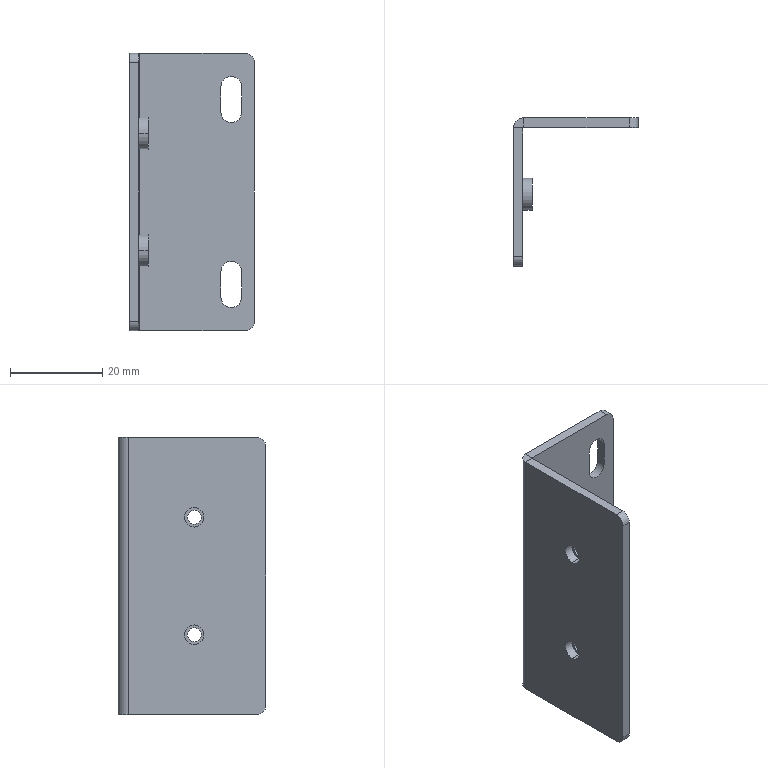Part | STEP file | FBDS-BJ-015 | 1 solid | 44 faces | box 27 x 32 x 60 mm | volume 6673 mm3 | cylinder 24 | plane 20 | commonest cylinder face diameters 4.5 x6 3 x4 4 x4 4.2 x4 6.87 x4 0.4 x1
STEP:
#1=CARTESIAN_POINT('',(2.,-13.,-12.7));
#2=VERTEX_POINT('',#1);
#3=CARTESIAN_POINT('',(2.,-16.,-12.7));
#4=VERTEX_POINT('',#3);
#5=CARTESIAN_POINT('',(2.,-14.5,-12.7));
#6=DIRECTION('',(-1.,0.,0.));
#7=DIRECTION('',(0.,-1.,0.));
#8=AXIS2_PLACEMENT_3D('',#5,#6,#7);
#9=CIRCLE('',#8,1.5);
#10=EDGE_CURVE('',#2,#4,#9,.T.);
#11=ORIENTED_EDGE('',*,*,#10,.F.);
#12=CARTESIAN_POINT('',(0.,-13.,-12.7));
#13=VERTEX_POINT('',#12);
#14=CARTESIAN_POINT('',(2.,-13.,-12.7));
#15=DIRECTION('',(-1.,0.,0.));
#16=VECTOR('',#15,1000.);
#17=LINE('',#14,#16);
#18=EDGE_CURVE('',#2,#13,#17,.T.);
#19=ORIENTED_EDGE('',*,*,#18,.T.);
#20=CARTESIAN_POINT('',(0.,-16.,-12.7));
#21=VERTEX_POINT('',#20);
#22=CARTESIAN_POINT('',(0.,-14.5,-12.7));
#23=DIRECTION('',(-1.,0.,0.));
#24=DIRECTION('',(0.,-1.,0.));
#25=AXIS2_PLACEMENT_3D('',#22,#23,#24);
#26=CIRCLE('',#25,1.5);
#27=EDGE_CURVE('',#13,#21,#26,.T.);
#28=ORIENTED_EDGE('',*,*,#27,.T.);
#29=CARTESIAN_POINT('',(2.,-16.,-12.7));
#30=DIRECTION('',(-1.,0.,0.));
#31=VECTOR('',#30,1000.);
#32=LINE('',#29,#31);
#33=EDGE_CURVE('',#4,#21,#32,.T.);
#34=ORIENTED_EDGE('',*,*,#33,.F.);
#35=EDGE_LOOP('',(#11,#19,#28,#34));
#36=FACE_OUTER_BOUND('',#35,.T.);
#37=CARTESIAN_POINT('',(2.,-14.5,-12.7));
#38=DIRECTION('',(-1.,0.,0.));
#39=DIRECTION('',(0.,-1.,0.));
#40=AXIS2_PLACEMENT_3D('',#37,#38,#39);
#41=CYLINDRICAL_SURFACE('',#40,1.5);
#42=ADVANCED_FACE('',(#36),#41,.F.);
#43=CARTESIAN_POINT('',(2.,-17.935,-12.7));
#44=VERTEX_POINT('',#43);
#45=CARTESIAN_POINT('',(2.,-11.065,-12.7));
#46=VERTEX_POINT('',#45);
#47=CARTESIAN_POINT('',(2.,-14.5,-12.7));
#48=DIRECTION('',(-1.,0.,0.));
#49=DIRECTION('',(0.,0.,1.));
#50=AXIS2_PLACEMENT_3D('',#47,#48,#49);
#51=CIRCLE('',#50,3.435);
#52=EDGE_CURVE('',#44,#46,#51,.T.);
#53=ORIENTED_EDGE('',*,*,#52,.T.);
#54=CARTESIAN_POINT('',(0.,-11.065,-12.7));
#55=VERTEX_POINT('',#54);
#56=CARTESIAN_POINT('',(2.,-11.065,-12.7));
#57=DIRECTION('',(-1.,0.,0.));
#58=VECTOR('',#57,1000.);
#59=LINE('',#56,#58);
#60=EDGE_CURVE('',#46,#55,#59,.T.);
#61=ORIENTED_EDGE('',*,*,#60,.T.);
#62=CARTESIAN_POINT('',(0.,-17.935,-12.7));
#63=VERTEX_POINT('',#62);
#64=CARTESIAN_POINT('',(0.,-14.5,-12.7));
#65=DIRECTION('',(1.,0.,0.));
#66=DIRECTION('',(0.,1.,0.));
#67=AXIS2_PLACEMENT_3D('',#64,#65,#66);
#68=CIRCLE('',#67,3.435);
#69=EDGE_CURVE('',#55,#63,#68,.T.);
#70=ORIENTED_EDGE('',*,*,#69,.T.);
#71=CARTESIAN_POINT('',(2.,-17.935,-12.7));
#72=DIRECTION('',(-1.,0.,0.));
#73=VECTOR('',#72,1000.);
#74=LINE('',#71,#73);
#75=EDGE_CURVE('',#44,#63,#74,.T.);
#76=ORIENTED_EDGE('',*,*,#75,.F.);
#77=EDGE_LOOP('',(#53,#61,#70,#76));
#78=FACE_OUTER_BOUND('',#77,.T.);
#79=CARTESIAN_POINT('',(2.,-14.5,-12.7));
#80=DIRECTION('',(-1.,0.,0.));
#81=DIRECTION('',(0.,-1.,0.));
#82=AXIS2_PLACEMENT_3D('',#79,#80,#81);
#83=CYLINDRICAL_SURFACE('',#82,3.435);
#84=ADVANCED_FACE('',(#78),#83,.T.);
#85=CARTESIAN_POINT('',(2.,-13.,12.7));
#86=VERTEX_POINT('',#85);
#87=CARTESIAN_POINT('',(2.,-16.,12.7));
#88=VERTEX_POINT('',#87);
#89=CARTESIAN_POINT('',(2.,-14.5,12.7));
#90=DIRECTION('',(-1.,0.,0.));
#91=DIRECTION('',(0.,-1.,0.));
#92=AXIS2_PLACEMENT_3D('',#89,#90,#91);
#93=CIRCLE('',#92,1.5);
#94=EDGE_CURVE('',#86,#88,#93,.T.);
#95=ORIENTED_EDGE('',*,*,#94,.F.);
#96=CARTESIAN_POINT('',(0.,-13.,12.7));
#97=VERTEX_POINT('',#96);
#98=CARTESIAN_POINT('',(2.,-13.,12.7));
#99=DIRECTION('',(-1.,0.,0.));
#100=VECTOR('',#99,1000.);
#101=LINE('',#98,#100);
#102=EDGE_CURVE('',#86,#97,#101,.T.);
#103=ORIENTED_EDGE('',*,*,#102,.T.);
#104=CARTESIAN_POINT('',(0.,-16.,12.7));
#105=VERTEX_POINT('',#104);
#106=CARTESIAN_POINT('',(0.,-14.5,12.7));
#107=DIRECTION('',(-1.,0.,0.));
#108=DIRECTION('',(0.,-1.,0.));
#109=AXIS2_PLACEMENT_3D('',#106,#107,#108);
#110=CIRCLE('',#109,1.5);
#111=EDGE_CURVE('',#97,#105,#110,.T.);
#112=ORIENTED_EDGE('',*,*,#111,.T.);
#113=CARTESIAN_POINT('',(2.,-16.,12.7));
#114=DIRECTION('',(-1.,0.,0.));
#115=VECTOR('',#114,1000.);
#116=LINE('',#113,#115);
#117=EDGE_CURVE('',#88,#105,#116,.T.);
#118=ORIENTED_EDGE('',*,*,#117,.F.);
#119=EDGE_LOOP('',(#95,#103,#112,#118));
#120=FACE_OUTER_BOUND('',#119,.T.);
#121=CARTESIAN_POINT('',(2.,-14.5,12.7));
#122=DIRECTION('',(-1.,0.,0.));
#123=DIRECTION('',(0.,-1.,0.));
#124=AXIS2_PLACEMENT_3D('',#121,#122,#123);
#125=CYLINDRICAL_SURFACE('',#124,1.5);
#126=ADVANCED_FACE('',(#120),#125,.F.);
#127=CARTESIAN_POINT('',(2.,-17.935,12.7));
#128=VERTEX_POINT('',#127);
#129=CARTESIAN_POINT('',(2.,-11.065,12.7));
#130=VERTEX_POINT('',#129);
#131=CARTESIAN_POINT('',(2.,-14.5,12.7));
#132=DIRECTION('',(-1.,0.,0.));
#133=DIRECTION('',(0.,0.,1.));
#134=AXIS2_PLACEMENT_3D('',#131,#132,#133);
#135=CIRCLE('',#134,3.435);
#136=EDGE_CURVE('',#128,#130,#135,.T.);
#137=ORIENTED_EDGE('',*,*,#136,.T.);
#138=CARTESIAN_POINT('',(0.,-11.065,12.7));
#139=VERTEX_POINT('',#138);
#140=CARTESIAN_POINT('',(2.,-11.065,12.7));
#141=DIRECTION('',(-1.,0.,0.));
#142=VECTOR('',#141,1000.);
#143=LINE('',#140,#142);
#144=EDGE_CURVE('',#130,#139,#143,.T.);
#145=ORIENTED_EDGE('',*,*,#144,.T.);
#146=CARTESIAN_POINT('',(0.,-17.935,12.7));
#147=VERTEX_POINT('',#146);
#148=CARTESIAN_POINT('',(0.,-14.5,12.7));
#149=DIRECTION('',(1.,0.,0.));
#150=DIRECTION('',(0.,1.,0.));
#151=AXIS2_PLACEMENT_3D('',#148,#149,#150);
#152=CIRCLE('',#151,3.435);
#153=EDGE_CURVE('',#139,#147,#152,.T.);
#154=ORIENTED_EDGE('',*,*,#153,.T.);
#155=CARTESIAN_POINT('',(2.,-17.935,12.7));
#156=DIRECTION('',(-1.,0.,0.));
#157=VECTOR('',#156,1000.);
#158=LINE('',#155,#157);
#159=EDGE_CURVE('',#128,#147,#158,.T.);
#160=ORIENTED_EDGE('',*,*,#159,.F.);
#161=EDGE_LOOP('',(#137,#145,#154,#160));
#162=FACE_OUTER_BOUND('',#161,.T.);
#163=CARTESIAN_POINT('',(2.,-14.5,12.7));
#164=DIRECTION('',(-1.,0.,0.));
#165=DIRECTION('',(0.,-1.,0.));
#166=AXIS2_PLACEMENT_3D('',#163,#164,#165);
#167=CYLINDRICAL_SURFACE('',#166,3.435);
#168=ADVANCED_FACE('',(#162),#167,.T.);
#169=CARTESIAN_POINT('',(22.25,0.,22.75));
#170=VERTEX_POINT('',#169);
#171=CARTESIAN_POINT('',(20.,0.,25.));
#172=VERTEX_POINT('',#171);
#173=CARTESIAN_POINT('',(20.,0.,22.75));
#174=DIRECTION('',(0.,-1.,0.));
#175=DIRECTION('',(0.,0.,-1.));
#176=AXIS2_PLACEMENT_3D('',#173,#174,#175);
#177=CIRCLE('',#176,2.25);
#178=EDGE_CURVE('',#170,#172,#177,.T.);
#179=ORIENTED_EDGE('',*,*,#178,.T.);
#180=CARTESIAN_POINT('',(20.,2.,25.));
#181=VERTEX_POINT('',#180);
#182=CARTESIAN_POINT('',(20.,2.,25.));
#183=DIRECTION('',(0.,1.,0.));
#184=VECTOR('',#183,1000.);
#185=LINE('',#182,#184);
#186=EDGE_CURVE('',#172,#181,#185,.T.);
#187=ORIENTED_EDGE('',*,*,#186,.T.);
#188=CARTESIAN_POINT('',(22.25,2.,22.75));
#189=VERTEX_POINT('',#188);
#190=CARTESIAN_POINT('',(20.,2.,22.75));
#191=DIRECTION('',(0.,1.,0.));
#192=DIRECTION('',(0.,0.,1.));
#193=AXIS2_PLACEMENT_3D('',#190,#191,#192);
#194=CIRCLE('',#193,2.25);
#195=EDGE_CURVE('',#181,#189,#194,.T.);
#196=ORIENTED_EDGE('',*,*,#195,.T.);
#197=CARTESIAN_POINT('',(22.25,-8.1,22.75));
#198=DIRECTION('',(0.,-1.,0.));
#199=VECTOR('',#198,1000.);
#200=LINE('',#197,#199);
#201=EDGE_CURVE('',#189,#170,#200,.T.);
#202=ORIENTED_EDGE('',*,*,#201,.T.);
#203=EDGE_LOOP('',(#179,#187,#196,#202));
#204=FACE_OUTER_BOUND('',#203,.T.);
#205=CARTESIAN_POINT('',(20.,2.,22.75));
#206=DIRECTION('',(0.,1.,0.));
#207=DIRECTION('',(0.,0.,1.));
#208=AXIS2_PLACEMENT_3D('',#205,#206,#207);
#209=CYLINDRICAL_SURFACE('',#208,2.25);
#210=ADVANCED_FACE('',(#204),#209,.F.);
#211=CARTESIAN_POINT('',(22.25,0.,-17.25));
#212=VERTEX_POINT('',#211);
#213=CARTESIAN_POINT('',(20.,0.,-15.));
#214=VERTEX_POINT('',#213);
#215=CARTESIAN_POINT('',(20.,0.,-17.25));
#216=DIRECTION('',(0.,-1.,0.));
#217=DIRECTION('',(0.,0.,-1.));
#218=AXIS2_PLACEMENT_3D('',#215,#216,#217);
#219=CIRCLE('',#218,2.25);
#220=EDGE_CURVE('',#212,#214,#219,.T.);
#221=ORIENTED_EDGE('',*,*,#220,.T.);
#222=CARTESIAN_POINT('',(20.,2.,-15.));
#223=VERTEX_POINT('',#222);
#224=CARTESIAN_POINT('',(20.,2.,-15.));
#225=DIRECTION('',(0.,1.,0.));
#226=VECTOR('',#225,1000.);
#227=LINE('',#224,#226);
#228=EDGE_CURVE('',#214,#223,#227,.T.);
#229=ORIENTED_EDGE('',*,*,#228,.T.);
#230=CARTESIAN_POINT('',(22.25,2.,-17.25));
#231=VERTEX_POINT('',#230);
#232=CARTESIAN_POINT('',(20.,2.,-17.25));
#233=DIRECTION('',(0.,1.,0.));
#234=DIRECTION('',(0.,0.,1.));
#235=AXIS2_PLACEMENT_3D('',#232,#233,#234);
#236=CIRCLE('',#235,2.25);
#237=EDGE_CURVE('',#223,#231,#236,.T.);
#238=ORIENTED_EDGE('',*,*,#237,.T.);
#239=CARTESIAN_POINT('',(22.25,-8.1,-17.25));
#240=DIRECTION('',(0.,-1.,0.));
#241=VECTOR('',#240,1000.);
#242=LINE('',#239,#241);
#243=EDGE_CURVE('',#231,#212,#242,.T.);
#244=ORIENTED_EDGE('',*,*,#243,.T.);
#245=EDGE_LOOP('',(#221,#229,#238,#244));
#246=FACE_OUTER_BOUND('',#245,.T.);
#247=CARTESIAN_POINT('',(20.,2.,-17.25));
#248=DIRECTION('',(0.,1.,0.));
#249=DIRECTION('',(0.,0.,1.));
#250=AXIS2_PLACEMENT_3D('',#247,#248,#249);
#251=CYLINDRICAL_SURFACE('',#250,2.25);
#252=ADVANCED_FACE('',(#246),#251,.F.);
#253=CARTESIAN_POINT('',(0.,-14.5,14.8));
#254=VERTEX_POINT('',#253);
#255=CARTESIAN_POINT('',(0.,-14.5,10.6));
#256=VERTEX_POINT('',#255);
#257=CARTESIAN_POINT('',(0.,-14.5,12.7));
#258=DIRECTION('',(1.,0.,0.));
#259=DIRECTION('',(0.,-1.,0.));
#260=AXIS2_PLACEMENT_3D('',#257,#258,#259);
#261=CIRCLE('',#260,2.1);
#262=EDGE_CURVE('',#254,#256,#261,.T.);
#263=ORIENTED_EDGE('',*,*,#262,.T.);
#264=CARTESIAN_POINT('',(-2.,-14.5,10.6));
#265=VERTEX_POINT('',#264);
#266=CARTESIAN_POINT('',(-2.,-14.5,10.6));
#267=DIRECTION('',(-1.,0.,0.));
#268=VECTOR('',#267,1000.);
#269=LINE('',#266,#268);
#270=EDGE_CURVE('',#256,#265,#269,.T.);
#271=ORIENTED_EDGE('',*,*,#270,.T.);
#272=CARTESIAN_POINT('',(-2.,-14.5,14.8));
#273=VERTEX_POINT('',#272);
#274=CARTESIAN_POINT('',(-2.,-14.5,12.7));
#275=DIRECTION('',(-1.,0.,0.));
#276=DIRECTION('',(0.,0.,1.));
#277=AXIS2_PLACEMENT_3D('',#274,#275,#276);
#278=CIRCLE('',#277,2.1);
#279=EDGE_CURVE('',#265,#273,#278,.T.);
#280=ORIENTED_EDGE('',*,*,#279,.T.);
#281=CARTESIAN_POINT('',(-2.,-14.5,14.8));
#282=DIRECTION('',(-1.,0.,0.));
#283=VECTOR('',#282,1000.);
#284=LINE('',#281,#283);
#285=EDGE_CURVE('',#254,#273,#284,.T.);
#286=ORIENTED_EDGE('',*,*,#285,.F.);
#287=EDGE_LOOP('',(#263,#271,#280,#286));
#288=FACE_OUTER_BOUND('',#287,.T.);
#289=CARTESIAN_POINT('',(-2.,-14.5,12.7));
#290=DIRECTION('',(-1.,0.,0.));
#291=DIRECTION('',(0.,0.,1.));
#292=AXIS2_PLACEMENT_3D('',#289,#290,#291);
#293=CYLINDRICAL_SURFACE('',#292,2.1);
#294=ADVANCED_FACE('',(#288),#293,.F.);
#295=CARTESIAN_POINT('',(0.,-14.5,-10.6));
#296=VERTEX_POINT('',#295);
#297=CARTESIAN_POINT('',(0.,-14.5,-14.8));
#298=VERTEX_POINT('',#297);
#299=CARTESIAN_POINT('',(0.,-14.5,-12.7));
#300=DIRECTION('',(1.,0.,0.));
#301=DIRECTION('',(0.,-1.,0.));
#302=AXIS2_PLACEMENT_3D('',#299,#300,#301);
#303=CIRCLE('',#302,2.1);
#304=EDGE_CURVE('',#296,#298,#303,.T.);
#305=ORIENTED_EDGE('',*,*,#304,.T.);
#306=CARTESIAN_POINT('',(-2.,-14.5,-14.8));
#307=VERTEX_POINT('',#306);
#308=CARTESIAN_POINT('',(-2.,-14.5,-14.8));
#309=DIRECTION('',(-1.,0.,0.));
#310=VECTOR('',#309,1000.);
#311=LINE('',#308,#310);
#312=EDGE_CURVE('',#298,#307,#311,.T.);
#313=ORIENTED_EDGE('',*,*,#312,.T.);
#314=CARTESIAN_POINT('',(-2.,-14.5,-10.6));
#315=VERTEX_POINT('',#314);
#316=CARTESIAN_POINT('',(-2.,-14.5,-12.7));
#317=DIRECTION('',(-1.,0.,0.));
#318=DIRECTION('',(0.,0.,1.));
#319=AXIS2_PLACEMENT_3D('',#316,#317,#318);
#320=CIRCLE('',#319,2.1);
#321=EDGE_CURVE('',#307,#315,#320,.T.);
#322=ORIENTED_EDGE('',*,*,#321,.T.);
#323=CARTESIAN_POINT('',(-2.,-14.5,-10.6));
#324=DIRECTION('',(-1.,0.,0.));
#325=VECTOR('',#324,1000.);
#326=LINE('',#323,#325);
#327=EDGE_CURVE('',#296,#315,#326,.T.);
#328=ORIENTED_EDGE('',*,*,#327,.F.);
#329=EDGE_LOOP('',(#305,#313,#322,#328));
#330=FACE_OUTER_BOUND('',#329,.T.);
#331=CARTESIAN_POINT('',(-2.,-14.5,-12.7));
#332=DIRECTION('',(-1.,0.,0.));
#333=DIRECTION('',(0.,0.,1.));
#334=AXIS2_PLACEMENT_3D('',#331,#332,#333);
#335=CYLINDRICAL_SURFACE('',#334,2.1);
#336=ADVANCED_FACE('',(#330),#335,.F.);
#337=CARTESIAN_POINT('',(17.75,2.,22.75));
#338=VERTEX_POINT('',#337);
#339=CARTESIAN_POINT('',(17.75,2.,17.25));
#340=VERTEX_POINT('',#339);
#341=CARTESIAN_POINT('',(17.75,2.,22.75));
#342=DIRECTION('',(0.,0.,-1.));
#343=VECTOR('',#342,1000.);
#344=LINE('',#341,#343);
#345=EDGE_CURVE('',#338,#340,#344,.T.);
#346=ORIENTED_EDGE('',*,*,#345,.T.);
#347=CARTESIAN_POINT('',(22.25,2.,17.25));
#348=VERTEX_POINT('',#347);
#349=CARTESIAN_POINT('',(20.,2.,17.25));
#350=DIRECTION('',(0.,1.,0.));
#351=DIRECTION('',(0.,0.,1.));
#352=AXIS2_PLACEMENT_3D('',#349,#350,#351);
#353=CIRCLE('',#352,2.25);
#354=EDGE_CURVE('',#348,#340,#353,.T.);
#355=ORIENTED_EDGE('',*,*,#354,.F.);
#356=CARTESIAN_POINT('',(22.25,2.,22.75));
#357=DIRECTION('',(0.,0.,-1.));
#358=VECTOR('',#357,1000.);
#359=LINE('',#356,#358);
#360=EDGE_CURVE('',#189,#348,#359,.T.);
#361=ORIENTED_EDGE('',*,*,#360,.F.);
#362=ORIENTED_EDGE('',*,*,#195,.F.);
#363=CARTESIAN_POINT('',(20.,2.,22.75));
#364=DIRECTION('',(0.,1.,0.));
#365=DIRECTION('',(0.,0.,1.));
#366=AXIS2_PLACEMENT_3D('',#363,#364,#365);
#367=CIRCLE('',#366,2.25);
#368=EDGE_CURVE('',#338,#181,#367,.T.);
#369=ORIENTED_EDGE('',*,*,#368,.F.);
#370=EDGE_LOOP('',(#346,#355,#361,#362,#369));
#371=FACE_BOUND('',#370,.T.);
#372=CARTESIAN_POINT('',(25.,2.,28.));
#373=VERTEX_POINT('',#372);
#374=CARTESIAN_POINT('',(25.,2.,-28.));
#375=VERTEX_POINT('',#374);
#376=CARTESIAN_POINT('',(25.,2.,30.));
#377=DIRECTION('',(0.,0.,-1.));
#378=VECTOR('',#377,1000.);
#379=LINE('',#376,#378);
#380=EDGE_CURVE('',#373,#375,#379,.T.);
#381=ORIENTED_EDGE('',*,*,#380,.T.);
#382=CARTESIAN_POINT('',(23.,2.,-30.));
#383=VERTEX_POINT('',#382);
#384=CARTESIAN_POINT('',(23.,2.,-28.));
#385=DIRECTION('',(0.,1.,0.));
#386=DIRECTION('',(0.,0.,-1.));
#387=AXIS2_PLACEMENT_3D('',#384,#385,#386);
#388=CIRCLE('',#387,2.);
#389=EDGE_CURVE('',#375,#383,#388,.T.);
#390=ORIENTED_EDGE('',*,*,#389,.T.);
#391=CARTESIAN_POINT('',(0.2,2.,-30.));
#392=VERTEX_POINT('',#391);
#393=CARTESIAN_POINT('',(0.,2.,-30.));
#394=DIRECTION('',(-1.,0.,0.));
#395=VECTOR('',#394,1000.);
#396=LINE('',#393,#395);
#397=EDGE_CURVE('',#383,#392,#396,.T.);
#398=ORIENTED_EDGE('',*,*,#397,.T.);
#399=CARTESIAN_POINT('',(0.2,2.,30.));
#400=VERTEX_POINT('',#399);
#401=CARTESIAN_POINT('',(0.2,2.,30.));
#402=DIRECTION('',(0.,0.,-1.));
#403=VECTOR('',#402,1000.);
#404=LINE('',#401,#403);
#405=EDGE_CURVE('',#400,#392,#404,.T.);
#406=ORIENTED_EDGE('',*,*,#405,.F.);
#407=CARTESIAN_POINT('',(23.,2.,30.));
#408=VERTEX_POINT('',#407);
#409=CARTESIAN_POINT('',(0.,2.,30.));
#410=DIRECTION('',(-1.,0.,0.));
#411=VECTOR('',#410,1000.);
#412=LINE('',#409,#411);
#413=EDGE_CURVE('',#408,#400,#412,.T.);
#414=ORIENTED_EDGE('',*,*,#413,.F.);
#415=CARTESIAN_POINT('',(23.,2.,28.));
#416=DIRECTION('',(0.,1.,0.));
#417=DIRECTION('',(0.,0.,-1.));
#418=AXIS2_PLACEMENT_3D('',#415,#416,#417);
#419=CIRCLE('',#418,2.);
#420=EDGE_CURVE('',#408,#373,#419,.T.);
#421=ORIENTED_EDGE('',*,*,#420,.T.);
#422=EDGE_LOOP('',(#381,#390,#398,#406,#414,#421));
#423=FACE_OUTER_BOUND('',#422,.T.);
#424=CARTESIAN_POINT('',(22.25,2.,-22.75));
#425=VERTEX_POINT('',#424);
#426=CARTESIAN_POINT('',(17.75,2.,-22.75));
#427=VERTEX_POINT('',#426);
#428=CARTESIAN_POINT('',(20.,2.,-22.75));
#429=DIRECTION('',(0.,1.,0.));
#430=DIRECTION('',(0.,0.,1.));
#431=AXIS2_PLACEMENT_3D('',#428,#429,#430);
#432=CIRCLE('',#431,2.25);
#433=EDGE_CURVE('',#425,#427,#432,.T.);
#434=ORIENTED_EDGE('',*,*,#433,.F.);
#435=CARTESIAN_POINT('',(22.25,2.,-17.25));
#436=DIRECTION('',(0.,0.,-1.));
#437=VECTOR('',#436,1000.);
#438=LINE('',#435,#437);
#439=EDGE_CURVE('',#231,#425,#438,.T.);
#440=ORIENTED_EDGE('',*,*,#439,.F.);
#441=ORIENTED_EDGE('',*,*,#237,.F.);
#442=CARTESIAN_POINT('',(17.75,2.,-17.25));
#443=VERTEX_POINT('',#442);
#444=CARTESIAN_POINT('',(20.,2.,-17.25));
#445=DIRECTION('',(0.,1.,0.));
#446=DIRECTION('',(0.,0.,1.));
#447=AXIS2_PLACEMENT_3D('',#444,#445,#446);
#448=CIRCLE('',#447,2.25);
#449=EDGE_CURVE('',#443,#223,#448,.T.);
#450=ORIENTED_EDGE('',*,*,#449,.F.);
#451=CARTESIAN_POINT('',(17.75,2.,-17.25));
#452=DIRECTION('',(0.,0.,-1.));
#453=VECTOR('',#452,1000.);
#454=LINE('',#451,#453);
#455=EDGE_CURVE('',#443,#427,#454,.T.);
#456=ORIENTED_EDGE('',*,*,#455,.T.);
#457=EDGE_LOOP('',(#434,#440,#441,#450,#456));
#458=FACE_BOUND('',#457,.T.);
#459=CARTESIAN_POINT('',(0.,2.,30.));
#460=DIRECTION('',(0.,-1.,0.));
#461=DIRECTION('',(0.,0.,-1.));
#462=AXIS2_PLACEMENT_3D('',#459,#460,#461);
#463=PLANE('',#462);
#464=ADVANCED_FACE('',(#371,#423,#458),#463,.F.);
#465=CARTESIAN_POINT('',(0.,-0.2,30.));
#466=VERTEX_POINT('',#465);
#467=CARTESIAN_POINT('',(-2.,-0.2,30.));
#468=VERTEX_POINT('',#467);
#469=CARTESIAN_POINT('',(0.,-0.2,30.));
#470=DIRECTION('',(-1.,0.,0.));
#471=VECTOR('',#470,1000.);
#472=LINE('',#469,#471);
#473=EDGE_CURVE('',#466,#468,#472,.T.);
#474=ORIENTED_EDGE('',*,*,#473,.F.);
#475=CARTESIAN_POINT('',(0.2,0.,30.));
#476=VERTEX_POINT('',#475);
#477=CARTESIAN_POINT('',(0.2,-0.2,30.));
#478=DIRECTION('',(0.,0.,1.));
#479=DIRECTION('',(-1.,0.,0.));
#480=AXIS2_PLACEMENT_3D('',#477,#478,#479);
#481=CIRCLE('',#480,0.2);
#482=EDGE_CURVE('',#476,#466,#481,.T.);
#483=ORIENTED_EDGE('',*,*,#482,.F.);
#484=CARTESIAN_POINT('',(0.2,2.,30.));
#485=DIRECTION('',(0.,-1.,0.));
#486=VECTOR('',#485,1000.);
#487=LINE('',#484,#486);
#488=EDGE_CURVE('',#400,#476,#487,.T.);
#489=ORIENTED_EDGE('',*,*,#488,.F.);
#490=CARTESIAN_POINT('',(0.2,-0.2,30.));
#491=DIRECTION('',(0.,0.,1.));
#492=DIRECTION('',(1.,0.,0.));
#493=AXIS2_PLACEMENT_3D('',#490,#491,#492);
#494=CIRCLE('',#493,2.2);
#495=EDGE_CURVE('',#400,#468,#494,.T.);
#496=ORIENTED_EDGE('',*,*,#495,.T.);
#497=EDGE_LOOP('',(#474,#483,#489,#496));
#498=FACE_OUTER_BOUND('',#497,.T.);
#499=CARTESIAN_POINT('',(0.,-0.2,30.));
#500=DIRECTION('',(0.,0.,1.));
#501=DIRECTION('',(1.,0.,0.));
#502=AXIS2_PLACEMENT_3D('',#499,#500,#501);
#503=PLANE('',#502);
#504=ADVANCED_FACE('',(#498),#503,.T.);
#505=CARTESIAN_POINT('',(-2.,-28.,30.));
#506=VERTEX_POINT('',#505);
#507=CARTESIAN_POINT('',(-2.,0.,30.));
#508=DIRECTION('',(0.,-1.,0.));
#509=VECTOR('',#508,1000.);
#510=LINE('',#507,#509);
#511=EDGE_CURVE('',#468,#506,#510,.T.);
#512=ORIENTED_EDGE('',*,*,#511,.T.);
#513=CARTESIAN_POINT('',(0.,-28.,30.));
#514=VERTEX_POINT('',#513);
#515=CARTESIAN_POINT('',(0.2,-28.,30.));
#516=DIRECTION('',(1.,0.,0.));
#517=VECTOR('',#516,1000.);
#518=LINE('',#515,#517);
#519=EDGE_CURVE('',#506,#514,#518,.T.);
#520=ORIENTED_EDGE('',*,*,#519,.T.);
#521=CARTESIAN_POINT('',(0.,0.,30.));
#522=DIRECTION('',(0.,-1.,0.));
#523=VECTOR('',#522,1000.);
#524=LINE('',#521,#523);
#525=EDGE_CURVE('',#466,#514,#524,.T.);
#526=ORIENTED_EDGE('',*,*,#525,.F.);
#527=ORIENTED_EDGE('',*,*,#473,.T.);
#528=EDGE_LOOP('',(#512,#520,#526,#527));
#529=FACE_OUTER_BOUND('',#528,.T.);
#530=CARTESIAN_POINT('',(0.2,2.,30.));
#531=DIRECTION('',(0.,0.,1.));
#532=DIRECTION('',(1.,0.,0.));
#533=AXIS2_PLACEMENT_3D('',#530,#531,#532);
#534=PLANE('',#533);
#535=ADVANCED_FACE('',(#529),#534,.T.);
#536=CARTESIAN_POINT('',(0.2,0.,-30.));
#537=VERTEX_POINT('',#536);
#538=CARTESIAN_POINT('',(0.2,0.,-30.));
#539=DIRECTION('',(0.,1.,0.));
#540=VECTOR('',#539,1000.);
#541=LINE('',#538,#540);
#542=EDGE_CURVE('',#537,#392,#541,.T.);
#543=ORIENTED_EDGE('',*,*,#542,.F.);
#544=CARTESIAN_POINT('',(0.,-0.2,-30.));
#545=VERTEX_POINT('',#544);
#546=CARTESIAN_POINT('',(0.2,-0.2,-30.));
#547=DIRECTION('',(0.,0.,1.));
#548=DIRECTION('',(-1.,0.,0.));
#549=AXIS2_PLACEMENT_3D('',#546,#547,#548);
#550=CIRCLE('',#549,0.2);
#551=EDGE_CURVE('',#537,#545,#550,.T.);
#552=ORIENTED_EDGE('',*,*,#551,.T.);
#553=CARTESIAN_POINT('',(-2.,-0.2,-30.));
#554=VERTEX_POINT('',#553);
#555=CARTESIAN_POINT('',(-2.,-0.2,-30.));
#556=DIRECTION('',(1.,0.,0.));
#557=VECTOR('',#556,1000.);
#558=LINE('',#555,#557);
#559=EDGE_CURVE('',#554,#545,#558,.T.);
#560=ORIENTED_EDGE('',*,*,#559,.F.);
#561=CARTESIAN_POINT('',(0.2,-0.2,-30.));
#562=DIRECTION('',(0.,0.,1.));
#563=DIRECTION('',(1.,0.,0.));
#564=AXIS2_PLACEMENT_3D('',#561,#562,#563);
#565=CIRCLE('',#564,2.2);
#566=EDGE_CURVE('',#392,#554,#565,.T.);
#567=ORIENTED_EDGE('',*,*,#566,.F.);
#568=EDGE_LOOP('',(#543,#552,#560,#567));
#569=FACE_OUTER_BOUND('',#568,.T.);
#570=CARTESIAN_POINT('',(0.2,0.,-30.));
#571=DIRECTION('',(0.,0.,-1.));
#572=DIRECTION('',(-1.,0.,0.));
#573=AXIS2_PLACEMENT_3D('',#570,#571,#572);
#574=PLANE('',#573);
#575=ADVANCED_FACE('',(#569),#574,.T.);
#576=ORIENTED_EDGE('',*,*,#397,.F.);
#577=CARTESIAN_POINT('',(23.,0.,-30.));
#578=VERTEX_POINT('',#577);
#579=CARTESIAN_POINT('',(23.,-0.2,-30.));
#580=DIRECTION('',(0.,-1.,0.));
#581=VECTOR('',#580,1000.);
#582=LINE('',#579,#581);
#583=EDGE_CURVE('',#383,#578,#582,.T.);
#584=ORIENTED_EDGE('',*,*,#583,.T.);
#585=CARTESIAN_POINT('',(0.,0.,-30.));
#586=DIRECTION('',(-1.,0.,0.));
#587=VECTOR('',#586,1000.);
#588=LINE('',#585,#587);
#589=EDGE_CURVE('',#578,#537,#588,.T.);
#590=ORIENTED_EDGE('',*,*,#589,.T.);
#591=ORIENTED_EDGE('',*,*,#542,.T.);
#592=EDGE_LOOP('',(#576,#584,#590,#591));
#593=FACE_OUTER_BOUND('',#592,.T.);
#594=CARTESIAN_POINT('',(-2.,-0.2,-30.));
#595=DIRECTION('',(0.,0.,-1.));
#596=DIRECTION('',(-1.,0.,0.));
#597=AXIS2_PLACEMENT_3D('',#594,#595,#596);
#598=PLANE('',#597);
#599=ADVANCED_FACE('',(#593),#598,.T.);
#600=CARTESIAN_POINT('',(-2.,-14.5,12.7));
#601=DIRECTION('',(-1.,0.,0.));
#602=DIRECTION('',(0.,0.,1.));
#603=AXIS2_PLACEMENT_3D('',#600,#601,#602);
#604=CIRCLE('',#603,2.1);
#605=EDGE_CURVE('',#273,#265,#604,.T.);
#606=ORIENTED_EDGE('',*,*,#605,.F.);
#607=ORIENTED_EDGE('',*,*,#279,.F.);
#608=EDGE_LOOP('',(#606,#607));
#609=FACE_BOUND('',#608,.T.);
#610=CARTESIAN_POINT('',(-2.,-14.5,-12.7));
#611=DIRECTION('',(-1.,0.,0.));
#612=DIRECTION('',(0.,0.,1.));
#613=AXIS2_PLACEMENT_3D('',#610,#611,#612);
#614=CIRCLE('',#613,2.1);
#615=EDGE_CURVE('',#315,#307,#614,.T.);
#616=ORIENTED_EDGE('',*,*,#615,.F.);
#617=ORIENTED_EDGE('',*,*,#321,.F.);
#618=EDGE_LOOP('',(#616,#617));
#619=FACE_BOUND('',#618,.T.);
#620=CARTESIAN_POINT('',(-2.,-28.,-30.));
#621=VERTEX_POINT('',#620);
#622=CARTESIAN_POINT('',(-2.,0.,-30.));
#623=DIRECTION('',(0.,-1.,0.));
#624=VECTOR('',#623,1000.);
#625=LINE('',#622,#624);
#626=EDGE_CURVE('',#554,#621,#625,.T.);
#627=ORIENTED_EDGE('',*,*,#626,.T.);
#628=CARTESIAN_POINT('',(-2.,-30.,-28.));
#629=VERTEX_POINT('',#628);
#630=CARTESIAN_POINT('',(-2.,-28.,-28.));
#631=DIRECTION('',(-1.,0.,0.));
#632=DIRECTION('',(0.,1.,0.));
#633=AXIS2_PLACEMENT_3D('',#630,#631,#632);
#634=CIRCLE('',#633,2.);
#635=EDGE_CURVE('',#621,#629,#634,.T.);
#636=ORIENTED_EDGE('',*,*,#635,.T.);
#637=CARTESIAN_POINT('',(-2.,-30.,28.));
#638=VERTEX_POINT('',#637);
#639=CARTESIAN_POINT('',(-2.,-30.,30.));
#640=DIRECTION('',(0.,0.,-1.));
#641=VECTOR('',#640,1000.);
#642=LINE('',#639,#641);
#643=EDGE_CURVE('',#638,#629,#642,.T.);
#644=ORIENTED_EDGE('',*,*,#643,.F.);
#645=CARTESIAN_POINT('',(-2.,-28.,28.));
#646=DIRECTION('',(-1.,0.,0.));
#647=DIRECTION('',(0.,1.,0.));
#648=AXIS2_PLACEMENT_3D('',#645,#646,#647);
#649=CIRCLE('',#648,2.);
#650=EDGE_CURVE('',#638,#506,#649,.T.);
#651=ORIENTED_EDGE('',*,*,#650,.T.);
#652=ORIENTED_EDGE('',*,*,#511,.F.);
#653=CARTESIAN_POINT('',(-2.,-0.2,30.));
#654=DIRECTION('',(0.,0.,-1.));
#655=VECTOR('',#654,1000.);
#656=LINE('',#653,#655);
#657=EDGE_CURVE('',#468,#554,#656,.T.);
#658=ORIENTED_EDGE('',*,*,#657,.T.);
#659=EDGE_LOOP('',(#627,#636,#644,#651,#652,#658));
#660=FACE_OUTER_BOUND('',#659,.T.);
#661=CARTESIAN_POINT('',(-2.,0.,30.));
#662=DIRECTION('',(1.,0.,0.));
#663=DIRECTION('',(0.,1.,0.));
#664=AXIS2_PLACEMENT_3D('',#661,#662,#663);
#665=PLANE('',#664);
#666=ADVANCED_FACE('',(#609,#619,#660),#665,.F.);
#667=ORIENTED_EDGE('',*,*,#643,.T.);
#668=CARTESIAN_POINT('',(0.,-30.,-28.));
#669=VERTEX_POINT('',#668);
#670=CARTESIAN_POINT('',(0.,-30.,-28.));
#671=DIRECTION('',(1.,0.,0.));
#672=VECTOR('',#671,1000.);
#673=LINE('',#670,#672);
#674=EDGE_CURVE('',#629,#669,#673,.T.);
#675=ORIENTED_EDGE('',*,*,#674,.T.);
#676=CARTESIAN_POINT('',(0.,-30.,28.));
#677=VERTEX_POINT('',#676);
#678=CARTESIAN_POINT('',(0.,-30.,30.));
#679=DIRECTION('',(0.,0.,-1.));
#680=VECTOR('',#679,1000.);
#681=LINE('',#678,#680);
#682=EDGE_CURVE('',#677,#669,#681,.T.);
#683=ORIENTED_EDGE('',*,*,#682,.F.);
#684=CARTESIAN_POINT('',(0.,-30.,28.));
#685=DIRECTION('',(-1.,0.,0.));
#686=VECTOR('',#685,1000.);
#687=LINE('',#684,#686);
#688=EDGE_CURVE('',#677,#638,#687,.T.);
#689=ORIENTED_EDGE('',*,*,#688,.T.);
#690=EDGE_LOOP('',(#667,#675,#683,#689));
#691=FACE_OUTER_BOUND('',#690,.T.);
#692=CARTESIAN_POINT('',(0.,-30.,30.));
#693=DIRECTION('',(0.,-1.,0.));
#694=DIRECTION('',(0.,0.,-1.));
#695=AXIS2_PLACEMENT_3D('',#692,#693,#694);
#696=PLANE('',#695);
#697=ADVANCED_FACE('',(#691),#696,.T.);
#698=CARTESIAN_POINT('',(0.,-14.5,-12.7));
#699=DIRECTION('',(1.,0.,0.));
#700=DIRECTION('',(0.,1.,0.));
#701=AXIS2_PLACEMENT_3D('',#698,#699,#700);
#702=CIRCLE('',#701,3.435);
#703=EDGE_CURVE('',#63,#55,#702,.T.);
#704=ORIENTED_EDGE('',*,*,#703,.F.);
#705=ORIENTED_EDGE('',*,*,#69,.F.);
#706=EDGE_LOOP('',(#704,#705));
#707=FACE_BOUND('',#706,.T.);
#708=CARTESIAN_POINT('',(0.,-14.5,12.7));
#709=DIRECTION('',(1.,0.,0.));
#710=DIRECTION('',(0.,1.,0.));
#711=AXIS2_PLACEMENT_3D('',#708,#709,#710);
#712=CIRCLE('',#711,3.435);
#713=EDGE_CURVE('',#147,#139,#712,.T.);
#714=ORIENTED_EDGE('',*,*,#713,.F.);
#715=ORIENTED_EDGE('',*,*,#153,.F.);
#716=EDGE_LOOP('',(#714,#715));
#717=FACE_BOUND('',#716,.T.);
#718=ORIENTED_EDGE('',*,*,#682,.T.);
#719=CARTESIAN_POINT('',(0.,-28.,-30.));
#720=VERTEX_POINT('',#719);
#721=CARTESIAN_POINT('',(0.,-28.,-28.));
#722=DIRECTION('',(1.,0.,0.));
#723=DIRECTION('',(0.,1.,0.));
#724=AXIS2_PLACEMENT_3D('',#721,#722,#723);
#725=CIRCLE('',#724,2.);
#726=EDGE_CURVE('',#669,#720,#725,.T.);
#727=ORIENTED_EDGE('',*,*,#726,.T.);
#728=CARTESIAN_POINT('',(0.,0.,-30.));
#729=DIRECTION('',(0.,-1.,0.));
#730=VECTOR('',#729,1000.);
#731=LINE('',#728,#730);
#732=EDGE_CURVE('',#545,#720,#731,.T.);
#733=ORIENTED_EDGE('',*,*,#732,.F.);
#734=CARTESIAN_POINT('',(0.,-0.2,30.));
#735=DIRECTION('',(0.,0.,-1.));
#736=VECTOR('',#735,1000.);
#737=LINE('',#734,#736);
#738=EDGE_CURVE('',#466,#545,#737,.T.);
#739=ORIENTED_EDGE('',*,*,#738,.F.);
#740=ORIENTED_EDGE('',*,*,#525,.T.);
#741=CARTESIAN_POINT('',(0.,-28.,28.));
#742=DIRECTION('',(1.,0.,0.));
#743=DIRECTION('',(0.,1.,0.));
#744=AXIS2_PLACEMENT_3D('',#741,#742,#743);
#745=CIRCLE('',#744,2.);
#746=EDGE_CURVE('',#514,#677,#745,.T.);
#747=ORIENTED_EDGE('',*,*,#746,.T.);
#748=EDGE_LOOP('',(#718,#727,#733,#739,#740,#747));
#749=FACE_OUTER_BOUND('',#748,.T.);
#750=CARTESIAN_POINT('',(0.,0.,30.));
#751=DIRECTION('',(1.,0.,0.));
#752=DIRECTION('',(0.,1.,0.));
#753=AXIS2_PLACEMENT_3D('',#750,#751,#752);
#754=PLANE('',#753);
#755=ADVANCED_FACE('',(#707,#717,#749),#754,.T.);
#756=ORIENTED_EDGE('',*,*,#551,.F.);
#757=CARTESIAN_POINT('',(0.2,0.,30.));
#758=DIRECTION('',(0.,0.,-1.));
#759=VECTOR('',#758,1000.);
#760=LINE('',#757,#759);
#761=EDGE_CURVE('',#476,#537,#760,.T.);
#762=ORIENTED_EDGE('',*,*,#761,.F.);
#763=ORIENTED_EDGE('',*,*,#482,.T.);
#764=ORIENTED_EDGE('',*,*,#738,.T.);
#765=EDGE_LOOP('',(#756,#762,#763,#764));
#766=FACE_OUTER_BOUND('',#765,.T.);
#767=CARTESIAN_POINT('',(0.2,-0.2,30.));
#768=DIRECTION('',(0.,0.,-1.));
#769=DIRECTION('',(-1.,0.,0.));
#770=AXIS2_PLACEMENT_3D('',#767,#768,#769);
#771=CYLINDRICAL_SURFACE('',#770,0.2);
#772=ADVANCED_FACE('',(#766),#771,.F.);
#773=CARTESIAN_POINT('',(17.75,0.,17.25));
#774=VERTEX_POINT('',#773);
#775=CARTESIAN_POINT('',(22.25,0.,17.25));
#776=VERTEX_POINT('',#775);
#777=CARTESIAN_POINT('',(20.,0.,17.25));
#778=DIRECTION('',(0.,-1.,0.));
#779=DIRECTION('',(0.,0.,-1.));
#780=AXIS2_PLACEMENT_3D('',#777,#778,#779);
#781=CIRCLE('',#780,2.25);
#782=EDGE_CURVE('',#774,#776,#781,.T.);
#783=ORIENTED_EDGE('',*,*,#782,.F.);
#784=CARTESIAN_POINT('',(17.75,0.,22.75));
#785=VERTEX_POINT('',#784);
#786=CARTESIAN_POINT('',(17.75,0.,70.));
#787=DIRECTION('',(0.,0.,-1.));
#788=VECTOR('',#787,1000.);
#789=LINE('',#786,#788);
#790=EDGE_CURVE('',#785,#774,#789,.T.);
#791=ORIENTED_EDGE('',*,*,#790,.F.);
#792=CARTESIAN_POINT('',(20.,0.,22.75));
#793=DIRECTION('',(0.,-1.,0.));
#794=DIRECTION('',(0.,0.,-1.));
#795=AXIS2_PLACEMENT_3D('',#792,#793,#794);
#796=CIRCLE('',#795,2.25);
#797=EDGE_CURVE('',#172,#785,#796,.T.);
#798=ORIENTED_EDGE('',*,*,#797,.F.);
#799=ORIENTED_EDGE('',*,*,#178,.F.);
#800=CARTESIAN_POINT('',(22.25,0.,70.));
#801=DIRECTION('',(0.,0.,1.));
#802=VECTOR('',#801,1000.);
#803=LINE('',#800,#802);
#804=EDGE_CURVE('',#776,#170,#803,.T.);
#805=ORIENTED_EDGE('',*,*,#804,.F.);
#806=EDGE_LOOP('',(#783,#791,#798,#799,#805));
#807=FACE_BOUND('',#806,.T.);
#808=CARTESIAN_POINT('',(17.75,0.,-17.25));
#809=VERTEX_POINT('',#808);
#810=CARTESIAN_POINT('',(17.75,0.,-22.75));
#811=VERTEX_POINT('',#810);
#812=CARTESIAN_POINT('',(17.75,0.,30.));
#813=DIRECTION('',(0.,0.,-1.));
#814=VECTOR('',#813,1000.);
#815=LINE('',#812,#814);
#816=EDGE_CURVE('',#809,#811,#815,.T.);
#817=ORIENTED_EDGE('',*,*,#816,.F.);
#818=CARTESIAN_POINT('',(20.,0.,-17.25));
#819=DIRECTION('',(0.,-1.,0.));
#820=DIRECTION('',(0.,0.,-1.));
#821=AXIS2_PLACEMENT_3D('',#818,#819,#820);
#822=CIRCLE('',#821,2.25);
#823=EDGE_CURVE('',#214,#809,#822,.T.);
#824=ORIENTED_EDGE('',*,*,#823,.F.);
#825=ORIENTED_EDGE('',*,*,#220,.F.);
#826=CARTESIAN_POINT('',(22.25,0.,-22.75));
#827=VERTEX_POINT('',#826);
#828=CARTESIAN_POINT('',(22.25,0.,30.));
#829=DIRECTION('',(0.,0.,1.));
#830=VECTOR('',#829,1000.);
#831=LINE('',#828,#830);
#832=EDGE_CURVE('',#827,#212,#831,.T.);
#833=ORIENTED_EDGE('',*,*,#832,.F.);
#834=CARTESIAN_POINT('',(20.,0.,-22.75));
#835=DIRECTION('',(0.,-1.,0.));
#836=DIRECTION('',(0.,0.,-1.));
#837=AXIS2_PLACEMENT_3D('',#834,#835,#836);
#838=CIRCLE('',#837,2.25);
#839=EDGE_CURVE('',#811,#827,#838,.T.);
#840=ORIENTED_EDGE('',*,*,#839,.F.);
#841=EDGE_LOOP('',(#817,#824,#825,#833,#840));
#842=FACE_BOUND('',#841,.T.);
#843=ORIENTED_EDGE('',*,*,#589,.F.);
#844=CARTESIAN_POINT('',(25.,0.,-28.));
#845=VERTEX_POINT('',#844);
#846=CARTESIAN_POINT('',(23.,0.,-28.));
#847=DIRECTION('',(0.,-1.,0.));
#848=DIRECTION('',(0.,0.,-1.));
#849=AXIS2_PLACEMENT_3D('',#846,#847,#848);
#850=CIRCLE('',#849,2.);
#851=EDGE_CURVE('',#578,#845,#850,.T.);
#852=ORIENTED_EDGE('',*,*,#851,.T.);
#853=CARTESIAN_POINT('',(25.,0.,28.));
#854=VERTEX_POINT('',#853);
#855=CARTESIAN_POINT('',(25.,0.,30.));
#856=DIRECTION('',(0.,0.,-1.));
#857=VECTOR('',#856,1000.);
#858=LINE('',#855,#857);
#859=EDGE_CURVE('',#854,#845,#858,.T.);
#860=ORIENTED_EDGE('',*,*,#859,.F.);
#861=CARTESIAN_POINT('',(23.,0.,30.));
#862=VERTEX_POINT('',#861);
#863=CARTESIAN_POINT('',(23.,0.,28.));
#864=DIRECTION('',(0.,-1.,0.));
#865=DIRECTION('',(0.,0.,-1.));
#866=AXIS2_PLACEMENT_3D('',#863,#864,#865);
#867=CIRCLE('',#866,2.);
#868=EDGE_CURVE('',#854,#862,#867,.T.);
#869=ORIENTED_EDGE('',*,*,#868,.T.);
#870=CARTESIAN_POINT('',(0.,0.,30.));
#871=DIRECTION('',(-1.,0.,0.));
#872=VECTOR('',#871,1000.);
#873=LINE('',#870,#872);
#874=EDGE_CURVE('',#862,#476,#873,.T.);
#875=ORIENTED_EDGE('',*,*,#874,.T.);
#876=ORIENTED_EDGE('',*,*,#761,.T.);
#877=EDGE_LOOP('',(#843,#852,#860,#869,#875,#876));
#878=FACE_OUTER_BOUND('',#877,.T.);
#879=CARTESIAN_POINT('',(0.,0.,30.));
#880=DIRECTION('',(0.,-1.,0.));
#881=DIRECTION('',(0.,0.,-1.));
#882=AXIS2_PLACEMENT_3D('',#879,#880,#881);
#883=PLANE('',#882);
#884=ADVANCED_FACE('',(#807,#842,#878),#883,.T.);
#885=ORIENTED_EDGE('',*,*,#859,.T.);
#886=CARTESIAN_POINT('',(25.,2.,-28.));
#887=DIRECTION('',(0.,1.,0.));
#888=VECTOR('',#887,1000.);
#889=LINE('',#886,#888);
#890=EDGE_CURVE('',#845,#375,#889,.T.);
#891=ORIENTED_EDGE('',*,*,#890,.T.);
#892=ORIENTED_EDGE('',*,*,#380,.F.);
#893=CARTESIAN_POINT('',(25.,0.,28.));
#894=DIRECTION('',(0.,-1.,0.));
#895=VECTOR('',#894,1000.);
#896=LINE('',#893,#895);
#897=EDGE_CURVE('',#373,#854,#896,.T.);
#898=ORIENTED_EDGE('',*,*,#897,.T.);
#899=EDGE_LOOP('',(#885,#891,#892,#898));
#900=FACE_OUTER_BOUND('',#899,.T.);
#901=CARTESIAN_POINT('',(25.,2.,30.));
#902=DIRECTION('',(1.,0.,0.));
#903=DIRECTION('',(0.,0.,-1.));
#904=AXIS2_PLACEMENT_3D('',#901,#902,#903);
#905=PLANE('',#904);
#906=ADVANCED_FACE('',(#900),#905,.T.);
#907=ORIENTED_EDGE('',*,*,#566,.T.);
#908=ORIENTED_EDGE('',*,*,#657,.F.);
#909=ORIENTED_EDGE('',*,*,#495,.F.);
#910=ORIENTED_EDGE('',*,*,#405,.T.);
#911=EDGE_LOOP('',(#907,#908,#909,#910));
#912=FACE_OUTER_BOUND('',#911,.T.);
#913=CARTESIAN_POINT('',(0.2,-0.2,30.));
#914=DIRECTION('',(0.,0.,-1.));
#915=DIRECTION('',(-1.,0.,0.));
#916=AXIS2_PLACEMENT_3D('',#913,#914,#915);
#917=CYLINDRICAL_SURFACE('',#916,2.2);
#918=ADVANCED_FACE('',(#912),#917,.T.);
#919=ORIENTED_EDGE('',*,*,#874,.F.);
#920=CARTESIAN_POINT('',(23.,2.,30.));
#921=DIRECTION('',(0.,1.,0.));
#922=VECTOR('',#921,1000.);
#923=LINE('',#920,#922);
#924=EDGE_CURVE('',#862,#408,#923,.T.);
#925=ORIENTED_EDGE('',*,*,#924,.T.);
#926=ORIENTED_EDGE('',*,*,#413,.T.);
#927=ORIENTED_EDGE('',*,*,#488,.T.);
#928=EDGE_LOOP('',(#919,#925,#926,#927));
#929=FACE_OUTER_BOUND('',#928,.T.);
#930=CARTESIAN_POINT('',(0.2,-0.2,30.));
#931=DIRECTION('',(0.,0.,-1.));
#932=DIRECTION('',(-1.,0.,0.));
#933=AXIS2_PLACEMENT_3D('',#930,#931,#932);
#934=PLANE('',#933);
#935=ADVANCED_FACE('',(#929),#934,.F.);
#936=ORIENTED_EDGE('',*,*,#732,.T.);
#937=CARTESIAN_POINT('',(0.2,-28.,-30.));
#938=DIRECTION('',(-1.,0.,0.));
#939=VECTOR('',#938,1000.);
#940=LINE('',#937,#939);
#941=EDGE_CURVE('',#720,#621,#940,.T.);
#942=ORIENTED_EDGE('',*,*,#941,.T.);
#943=ORIENTED_EDGE('',*,*,#626,.F.);
#944=ORIENTED_EDGE('',*,*,#559,.T.);
#945=EDGE_LOOP('',(#936,#942,#943,#944));
#946=FACE_OUTER_BOUND('',#945,.T.);
#947=CARTESIAN_POINT('',(0.2,-0.2,-30.));
#948=DIRECTION('',(0.,0.,-1.));
#949=DIRECTION('',(-1.,0.,0.));
#950=AXIS2_PLACEMENT_3D('',#947,#948,#949);
#951=PLANE('',#950);
#952=ADVANCED_FACE('',(#946),#951,.T.);
#953=ORIENTED_EDGE('',*,*,#312,.F.);
#954=CARTESIAN_POINT('',(0.,-14.5,-12.7));
#955=DIRECTION('',(1.,0.,0.));
#956=DIRECTION('',(0.,-1.,0.));
#957=AXIS2_PLACEMENT_3D('',#954,#955,#956);
#958=CIRCLE('',#957,2.1);
#959=EDGE_CURVE('',#298,#296,#958,.T.);
#960=ORIENTED_EDGE('',*,*,#959,.T.);
#961=ORIENTED_EDGE('',*,*,#327,.T.);
#962=ORIENTED_EDGE('',*,*,#615,.T.);
#963=EDGE_LOOP('',(#953,#960,#961,#962));
#964=FACE_OUTER_BOUND('',#963,.T.);
#965=CARTESIAN_POINT('',(-2.,-14.5,-12.7));
#966=DIRECTION('',(-1.,0.,0.));
#967=DIRECTION('',(0.,0.,1.));
#968=AXIS2_PLACEMENT_3D('',#965,#966,#967);
#969=CYLINDRICAL_SURFACE('',#968,2.1);
#970=ADVANCED_FACE('',(#964),#969,.F.);
#971=ORIENTED_EDGE('',*,*,#270,.F.);
#972=CARTESIAN_POINT('',(0.,-14.5,12.7));
#973=DIRECTION('',(1.,0.,0.));
#974=DIRECTION('',(0.,-1.,0.));
#975=AXIS2_PLACEMENT_3D('',#972,#973,#974);
#976=CIRCLE('',#975,2.1);
#977=EDGE_CURVE('',#256,#254,#976,.T.);
#978=ORIENTED_EDGE('',*,*,#977,.T.);
#979=ORIENTED_EDGE('',*,*,#285,.T.);
#980=ORIENTED_EDGE('',*,*,#605,.T.);
#981=EDGE_LOOP('',(#971,#978,#979,#980));
#982=FACE_OUTER_BOUND('',#981,.T.);
#983=CARTESIAN_POINT('',(-2.,-14.5,12.7));
#984=DIRECTION('',(-1.,0.,0.));
#985=DIRECTION('',(0.,0.,1.));
#986=AXIS2_PLACEMENT_3D('',#983,#984,#985);
#987=CYLINDRICAL_SURFACE('',#986,2.1);
#988=ADVANCED_FACE('',(#982),#987,.F.);
#989=ORIENTED_EDGE('',*,*,#839,.T.);
#990=CARTESIAN_POINT('',(22.25,-8.1,-22.75));
#991=DIRECTION('',(0.,-1.,0.));
#992=VECTOR('',#991,1000.);
#993=LINE('',#990,#992);
#994=EDGE_CURVE('',#425,#827,#993,.T.);
#995=ORIENTED_EDGE('',*,*,#994,.F.);
#996=ORIENTED_EDGE('',*,*,#433,.T.);
#997=CARTESIAN_POINT('',(17.75,2.,-22.75));
#998=DIRECTION('',(0.,1.,0.));
#999=VECTOR('',#998,1000.);
#1000=LINE('',#997,#999);
#1001=EDGE_CURVE('',#811,#427,#1000,.T.);
#1002=ORIENTED_EDGE('',*,*,#1001,.F.);
#1003=EDGE_LOOP('',(#989,#995,#996,#1002));
#1004=FACE_OUTER_BOUND('',#1003,.T.);
#1005=CARTESIAN_POINT('',(20.,2.,-22.75));
#1006=DIRECTION('',(0.,1.,0.));
#1007=DIRECTION('',(0.,0.,1.));
#1008=AXIS2_PLACEMENT_3D('',#1005,#1006,#1007);
#1009=CYLINDRICAL_SURFACE('',#1008,2.25);
#1010=ADVANCED_FACE('',(#1004),#1009,.F.);
#1011=ORIENTED_EDGE('',*,*,#228,.F.);
#1012=ORIENTED_EDGE('',*,*,#823,.T.);
#1013=CARTESIAN_POINT('',(17.75,2.,-17.25));
#1014=DIRECTION('',(0.,-1.,0.));
#1015=VECTOR('',#1014,1000.);
#1016=LINE('',#1013,#1015);
#1017=EDGE_CURVE('',#443,#809,#1016,.T.);
#1018=ORIENTED_EDGE('',*,*,#1017,.F.);
#1019=ORIENTED_EDGE('',*,*,#449,.T.);
#1020=EDGE_LOOP('',(#1011,#1012,#1018,#1019));
#1021=FACE_OUTER_BOUND('',#1020,.T.);
#1022=CARTESIAN_POINT('',(20.,2.,-17.25));
#1023=DIRECTION('',(0.,1.,0.));
#1024=DIRECTION('',(0.,0.,1.));
#1025=AXIS2_PLACEMENT_3D('',#1022,#1023,#1024);
#1026=CYLINDRICAL_SURFACE('',#1025,2.25);
#1027=ADVANCED_FACE('',(#1021),#1026,.F.);
#1028=ORIENTED_EDGE('',*,*,#816,.T.);
#1029=ORIENTED_EDGE('',*,*,#1001,.T.);
#1030=ORIENTED_EDGE('',*,*,#455,.F.);
#1031=ORIENTED_EDGE('',*,*,#1017,.T.);
#1032=EDGE_LOOP('',(#1028,#1029,#1030,#1031));
#1033=FACE_OUTER_BOUND('',#1032,.T.);
#1034=CARTESIAN_POINT('',(17.75,2.,-17.25));
#1035=DIRECTION('',(-1.,0.,0.));
#1036=DIRECTION('',(0.,0.,1.));
#1037=AXIS2_PLACEMENT_3D('',#1034,#1035,#1036);
#1038=PLANE('',#1037);
#1039=ADVANCED_FACE('',(#1033),#1038,.F.);
#1040=ORIENTED_EDGE('',*,*,#832,.T.);
#1041=ORIENTED_EDGE('',*,*,#243,.F.);
#1042=ORIENTED_EDGE('',*,*,#439,.T.);
#1043=ORIENTED_EDGE('',*,*,#994,.T.);
#1044=EDGE_LOOP('',(#1040,#1041,#1042,#1043));
#1045=FACE_OUTER_BOUND('',#1044,.T.);
#1046=CARTESIAN_POINT('',(22.25,-8.1,-17.25));
#1047=DIRECTION('',(1.,0.,0.));
#1048=DIRECTION('',(0.,1.,0.));
#1049=AXIS2_PLACEMENT_3D('',#1046,#1047,#1048);
#1050=PLANE('',#1049);
#1051=ADVANCED_FACE('',(#1045),#1050,.F.);
#1052=ORIENTED_EDGE('',*,*,#782,.T.);
#1053=CARTESIAN_POINT('',(22.25,-8.1,17.25));
#1054=DIRECTION('',(0.,-1.,0.));
#1055=VECTOR('',#1054,1000.);
#1056=LINE('',#1053,#1055);
#1057=EDGE_CURVE('',#348,#776,#1056,.T.);
#1058=ORIENTED_EDGE('',*,*,#1057,.F.);
#1059=ORIENTED_EDGE('',*,*,#354,.T.);
#1060=CARTESIAN_POINT('',(17.75,2.,17.25));
#1061=DIRECTION('',(0.,1.,0.));
#1062=VECTOR('',#1061,1000.);
#1063=LINE('',#1060,#1062);
#1064=EDGE_CURVE('',#774,#340,#1063,.T.);
#1065=ORIENTED_EDGE('',*,*,#1064,.F.);
#1066=EDGE_LOOP('',(#1052,#1058,#1059,#1065));
#1067=FACE_OUTER_BOUND('',#1066,.T.);
#1068=CARTESIAN_POINT('',(20.,2.,17.25));
#1069=DIRECTION('',(0.,1.,0.));
#1070=DIRECTION('',(0.,0.,1.));
#1071=AXIS2_PLACEMENT_3D('',#1068,#1069,#1070);
#1072=CYLINDRICAL_SURFACE('',#1071,2.25);
#1073=ADVANCED_FACE('',(#1067),#1072,.F.);
#1074=ORIENTED_EDGE('',*,*,#790,.T.);
#1075=ORIENTED_EDGE('',*,*,#1064,.T.);
#1076=ORIENTED_EDGE('',*,*,#345,.F.);
#1077=CARTESIAN_POINT('',(17.75,2.,22.75));
#1078=DIRECTION('',(0.,-1.,0.));
#1079=VECTOR('',#1078,1000.);
#1080=LINE('',#1077,#1079);
#1081=EDGE_CURVE('',#338,#785,#1080,.T.);
#1082=ORIENTED_EDGE('',*,*,#1081,.T.);
#1083=EDGE_LOOP('',(#1074,#1075,#1076,#1082));
#1084=FACE_OUTER_BOUND('',#1083,.T.);
#1085=CARTESIAN_POINT('',(17.75,2.,22.75));
#1086=DIRECTION('',(-1.,0.,0.));
#1087=DIRECTION('',(0.,0.,1.));
#1088=AXIS2_PLACEMENT_3D('',#1085,#1086,#1087);
#1089=PLANE('',#1088);
#1090=ADVANCED_FACE('',(#1084),#1089,.F.);
#1091=ORIENTED_EDGE('',*,*,#186,.F.);
#1092=ORIENTED_EDGE('',*,*,#797,.T.);
#1093=ORIENTED_EDGE('',*,*,#1081,.F.);
#1094=ORIENTED_EDGE('',*,*,#368,.T.);
#1095=EDGE_LOOP('',(#1091,#1092,#1093,#1094));
#1096=FACE_OUTER_BOUND('',#1095,.T.);
#1097=CARTESIAN_POINT('',(20.,2.,22.75));
#1098=DIRECTION('',(0.,1.,0.));
#1099=DIRECTION('',(0.,0.,1.));
#1100=AXIS2_PLACEMENT_3D('',#1097,#1098,#1099);
#1101=CYLINDRICAL_SURFACE('',#1100,2.25);
#1102=ADVANCED_FACE('',(#1096),#1101,.F.);
#1103=ORIENTED_EDGE('',*,*,#804,.T.);
#1104=ORIENTED_EDGE('',*,*,#201,.F.);
#1105=ORIENTED_EDGE('',*,*,#360,.T.);
#1106=ORIENTED_EDGE('',*,*,#1057,.T.);
#1107=EDGE_LOOP('',(#1103,#1104,#1105,#1106));
#1108=FACE_OUTER_BOUND('',#1107,.T.);
#1109=CARTESIAN_POINT('',(22.25,-8.1,22.75));
#1110=DIRECTION('',(1.,0.,0.));
#1111=DIRECTION('',(0.,1.,0.));
#1112=AXIS2_PLACEMENT_3D('',#1109,#1110,#1111);
#1113=PLANE('',#1112);
#1114=ADVANCED_FACE('',(#1108),#1113,.F.);
#1115=CARTESIAN_POINT('',(0.,-14.5,12.7));
#1116=DIRECTION('',(-1.,0.,0.));
#1117=DIRECTION('',(0.,-1.,0.));
#1118=AXIS2_PLACEMENT_3D('',#1115,#1116,#1117);
#1119=CIRCLE('',#1118,1.5);
#1120=EDGE_CURVE('',#105,#97,#1119,.T.);
#1121=ORIENTED_EDGE('',*,*,#1120,.F.);
#1122=ORIENTED_EDGE('',*,*,#111,.F.);
#1123=EDGE_LOOP('',(#1121,#1122));
#1124=FACE_BOUND('',#1123,.T.);
#1125=ORIENTED_EDGE('',*,*,#262,.F.);
#1126=ORIENTED_EDGE('',*,*,#977,.F.);
#1127=EDGE_LOOP('',(#1125,#1126));
#1128=FACE_OUTER_BOUND('',#1127,.T.);
#1129=CARTESIAN_POINT('',(0.,-14.5,12.7));
#1130=DIRECTION('',(-1.,0.,0.));
#1131=DIRECTION('',(0.,-1.,0.));
#1132=AXIS2_PLACEMENT_3D('',#1129,#1130,#1131);
#1133=PLANE('',#1132);
#1134=ADVANCED_FACE('',(#1124,#1128),#1133,.T.);
#1135=ORIENTED_EDGE('',*,*,#144,.F.);
#1136=CARTESIAN_POINT('',(2.,-14.5,12.7));
#1137=DIRECTION('',(-1.,0.,0.));
#1138=DIRECTION('',(0.,0.,1.));
#1139=AXIS2_PLACEMENT_3D('',#1136,#1137,#1138);
#1140=CIRCLE('',#1139,3.435);
#1141=EDGE_CURVE('',#130,#128,#1140,.T.);
#1142=ORIENTED_EDGE('',*,*,#1141,.T.);
#1143=ORIENTED_EDGE('',*,*,#159,.T.);
#1144=ORIENTED_EDGE('',*,*,#713,.T.);
#1145=EDGE_LOOP('',(#1135,#1142,#1143,#1144));
#1146=FACE_OUTER_BOUND('',#1145,.T.);
#1147=CARTESIAN_POINT('',(2.,-14.5,12.7));
#1148=DIRECTION('',(-1.,0.,0.));
#1149=DIRECTION('',(0.,-1.,0.));
#1150=AXIS2_PLACEMENT_3D('',#1147,#1148,#1149);
#1151=CYLINDRICAL_SURFACE('',#1150,3.435);
#1152=ADVANCED_FACE('',(#1146),#1151,.T.);
#1153=CARTESIAN_POINT('',(2.,-14.5,12.7));
#1154=DIRECTION('',(-1.,0.,0.));
#1155=DIRECTION('',(0.,-1.,0.));
#1156=AXIS2_PLACEMENT_3D('',#1153,#1154,#1155);
#1157=CIRCLE('',#1156,1.5);
#1158=EDGE_CURVE('',#88,#86,#1157,.T.);
#1159=ORIENTED_EDGE('',*,*,#1158,.T.);
#1160=ORIENTED_EDGE('',*,*,#94,.T.);
#1161=EDGE_LOOP('',(#1159,#1160));
#1162=FACE_BOUND('',#1161,.T.);
#1163=ORIENTED_EDGE('',*,*,#136,.F.);
#1164=ORIENTED_EDGE('',*,*,#1141,.F.);
#1165=EDGE_LOOP('',(#1163,#1164));
#1166=FACE_OUTER_BOUND('',#1165,.T.);
#1167=CARTESIAN_POINT('',(2.,-14.5,12.7));
#1168=DIRECTION('',(-1.,0.,0.));
#1169=DIRECTION('',(0.,-1.,0.));
#1170=AXIS2_PLACEMENT_3D('',#1167,#1168,#1169);
#1171=PLANE('',#1170);
#1172=ADVANCED_FACE('',(#1162,#1166),#1171,.F.);
#1173=ORIENTED_EDGE('',*,*,#102,.F.);
#1174=ORIENTED_EDGE('',*,*,#1158,.F.);
#1175=ORIENTED_EDGE('',*,*,#117,.T.);
#1176=ORIENTED_EDGE('',*,*,#1120,.T.);
#1177=EDGE_LOOP('',(#1173,#1174,#1175,#1176));
#1178=FACE_OUTER_BOUND('',#1177,.T.);
#1179=CARTESIAN_POINT('',(2.,-14.5,12.7));
#1180=DIRECTION('',(-1.,0.,0.));
#1181=DIRECTION('',(0.,-1.,0.));
#1182=AXIS2_PLACEMENT_3D('',#1179,#1180,#1181);
#1183=CYLINDRICAL_SURFACE('',#1182,1.5);
#1184=ADVANCED_FACE('',(#1178),#1183,.F.);
#1185=CARTESIAN_POINT('',(0.,-14.5,-12.7));
#1186=DIRECTION('',(-1.,0.,0.));
#1187=DIRECTION('',(0.,-1.,0.));
#1188=AXIS2_PLACEMENT_3D('',#1185,#1186,#1187);
#1189=CIRCLE('',#1188,1.5);
#1190=EDGE_CURVE('',#21,#13,#1189,.T.);
#1191=ORIENTED_EDGE('',*,*,#1190,.F.);
#1192=ORIENTED_EDGE('',*,*,#27,.F.);
#1193=EDGE_LOOP('',(#1191,#1192));
#1194=FACE_BOUND('',#1193,.T.);
#1195=ORIENTED_EDGE('',*,*,#304,.F.);
#1196=ORIENTED_EDGE('',*,*,#959,.F.);
#1197=EDGE_LOOP('',(#1195,#1196));
#1198=FACE_OUTER_BOUND('',#1197,.T.);
#1199=CARTESIAN_POINT('',(0.,-14.5,-12.7));
#1200=DIRECTION('',(-1.,0.,0.));
#1201=DIRECTION('',(0.,-1.,0.));
#1202=AXIS2_PLACEMENT_3D('',#1199,#1200,#1201);
#1203=PLANE('',#1202);
#1204=ADVANCED_FACE('',(#1194,#1198),#1203,.T.);
#1205=ORIENTED_EDGE('',*,*,#60,.F.);
#1206=CARTESIAN_POINT('',(2.,-14.5,-12.7));
#1207=DIRECTION('',(-1.,0.,0.));
#1208=DIRECTION('',(0.,0.,1.));
#1209=AXIS2_PLACEMENT_3D('',#1206,#1207,#1208);
#1210=CIRCLE('',#1209,3.435);
#1211=EDGE_CURVE('',#46,#44,#1210,.T.);
#1212=ORIENTED_EDGE('',*,*,#1211,.T.);
#1213=ORIENTED_EDGE('',*,*,#75,.T.);
#1214=ORIENTED_EDGE('',*,*,#703,.T.);
#1215=EDGE_LOOP('',(#1205,#1212,#1213,#1214));
#1216=FACE_OUTER_BOUND('',#1215,.T.);
#1217=CARTESIAN_POINT('',(2.,-14.5,-12.7));
#1218=DIRECTION('',(-1.,0.,0.));
#1219=DIRECTION('',(0.,-1.,0.));
#1220=AXIS2_PLACEMENT_3D('',#1217,#1218,#1219);
#1221=CYLINDRICAL_SURFACE('',#1220,3.435);
#1222=ADVANCED_FACE('',(#1216),#1221,.T.);
#1223=CARTESIAN_POINT('',(2.,-14.5,-12.7));
#1224=DIRECTION('',(-1.,0.,0.));
#1225=DIRECTION('',(0.,-1.,0.));
#1226=AXIS2_PLACEMENT_3D('',#1223,#1224,#1225);
#1227=CIRCLE('',#1226,1.5);
#1228=EDGE_CURVE('',#4,#2,#1227,.T.);
#1229=ORIENTED_EDGE('',*,*,#1228,.T.);
#1230=ORIENTED_EDGE('',*,*,#10,.T.);
#1231=EDGE_LOOP('',(#1229,#1230));
#1232=FACE_BOUND('',#1231,.T.);
#1233=ORIENTED_EDGE('',*,*,#52,.F.);
#1234=ORIENTED_EDGE('',*,*,#1211,.F.);
#1235=EDGE_LOOP('',(#1233,#1234));
#1236=FACE_OUTER_BOUND('',#1235,.T.);
#1237=CARTESIAN_POINT('',(2.,-14.5,-12.7));
#1238=DIRECTION('',(-1.,0.,0.));
#1239=DIRECTION('',(0.,-1.,0.));
#1240=AXIS2_PLACEMENT_3D('',#1237,#1238,#1239);
#1241=PLANE('',#1240);
#1242=ADVANCED_FACE('',(#1232,#1236),#1241,.F.);
#1243=ORIENTED_EDGE('',*,*,#18,.F.);
#1244=ORIENTED_EDGE('',*,*,#1228,.F.);
#1245=ORIENTED_EDGE('',*,*,#33,.T.);
#1246=ORIENTED_EDGE('',*,*,#1190,.T.);
#1247=EDGE_LOOP('',(#1243,#1244,#1245,#1246));
#1248=FACE_OUTER_BOUND('',#1247,.T.);
#1249=CARTESIAN_POINT('',(2.,-14.5,-12.7));
#1250=DIRECTION('',(-1.,0.,0.));
#1251=DIRECTION('',(0.,-1.,0.));
#1252=AXIS2_PLACEMENT_3D('',#1249,#1250,#1251);
#1253=CYLINDRICAL_SURFACE('',#1252,1.5);
#1254=ADVANCED_FACE('',(#1248),#1253,.F.);
#1255=ORIENTED_EDGE('',*,*,#726,.F.);
#1256=ORIENTED_EDGE('',*,*,#674,.F.);
#1257=ORIENTED_EDGE('',*,*,#635,.F.);
#1258=ORIENTED_EDGE('',*,*,#941,.F.);
#1259=EDGE_LOOP('',(#1255,#1256,#1257,#1258));
#1260=FACE_OUTER_BOUND('',#1259,.T.);
#1261=CARTESIAN_POINT('',(0.2,-28.,-28.));
#1262=DIRECTION('',(-1.,0.,0.));
#1263=DIRECTION('',(0.,0.,1.));
#1264=AXIS2_PLACEMENT_3D('',#1261,#1262,#1263);
#1265=CYLINDRICAL_SURFACE('',#1264,2.);
#1266=ADVANCED_FACE('',(#1260),#1265,.T.);
#1267=ORIENTED_EDGE('',*,*,#746,.F.);
#1268=ORIENTED_EDGE('',*,*,#519,.F.);
#1269=ORIENTED_EDGE('',*,*,#650,.F.);
#1270=ORIENTED_EDGE('',*,*,#688,.F.);
#1271=EDGE_LOOP('',(#1267,#1268,#1269,#1270));
#1272=FACE_OUTER_BOUND('',#1271,.T.);
#1273=CARTESIAN_POINT('',(0.,-28.,28.));
#1274=DIRECTION('',(-1.,0.,0.));
#1275=DIRECTION('',(0.,0.,1.));
#1276=AXIS2_PLACEMENT_3D('',#1273,#1274,#1275);
#1277=CYLINDRICAL_SURFACE('',#1276,2.);
#1278=ADVANCED_FACE('',(#1272),#1277,.T.);
#1279=ORIENTED_EDGE('',*,*,#389,.F.);
#1280=ORIENTED_EDGE('',*,*,#890,.F.);
#1281=ORIENTED_EDGE('',*,*,#851,.F.);
#1282=ORIENTED_EDGE('',*,*,#583,.F.);
#1283=EDGE_LOOP('',(#1279,#1280,#1281,#1282));
#1284=FACE_OUTER_BOUND('',#1283,.T.);
#1285=CARTESIAN_POINT('',(23.,-0.2,-28.));
#1286=DIRECTION('',(0.,-1.,0.));
#1287=DIRECTION('',(0.,0.,-1.));
#1288=AXIS2_PLACEMENT_3D('',#1285,#1286,#1287);
#1289=CYLINDRICAL_SURFACE('',#1288,2.);
#1290=ADVANCED_FACE('',(#1284),#1289,.T.);
#1291=ORIENTED_EDGE('',*,*,#420,.F.);
#1292=ORIENTED_EDGE('',*,*,#924,.F.);
#1293=ORIENTED_EDGE('',*,*,#868,.F.);
#1294=ORIENTED_EDGE('',*,*,#897,.F.);
#1295=EDGE_LOOP('',(#1291,#1292,#1293,#1294));
#1296=FACE_OUTER_BOUND('',#1295,.T.);
#1297=CARTESIAN_POINT('',(23.,2.,28.));
#1298=DIRECTION('',(0.,1.,0.));
#1299=DIRECTION('',(0.,0.,1.));
#1300=AXIS2_PLACEMENT_3D('',#1297,#1298,#1299);
#1301=CYLINDRICAL_SURFACE('',#1300,2.);
#1302=ADVANCED_FACE('',(#1296),#1301,.T.);
#1303=CLOSED_SHELL('',(#42,#84,#126,#168,#210,#252,#294,#336,#464,#504,#535,#575,#599,#666,#697,#755,#772,#884,#906,#918,#935,#952,#970,#988,#1010,#1027,#1039,#1051,#1073,#1090,#1102,#1114,#1134,#1152,#1172,#1184,#1204,#1222,#1242,#1254,#1266,#1278,#1290,#1302));
#1304=MANIFOLD_SOLID_BREP('',#1303);
#1305=CARTESIAN_POINT('',(0.,0.,0.));
#1306=DIRECTION('',(0.,0.,1.));
#1307=DIRECTION('',(1.,0.,0.));
#1308=AXIS2_PLACEMENT_3D('',#1305,#1306,#1307);
#1309=(LENGTH_UNIT()NAMED_UNIT(*)SI_UNIT(.MILLI.,.METRE.));
#1310=UNCERTAINTY_MEASURE_WITH_UNIT(LENGTH_MEASURE(0.00001),#1309,'','');
#1311=(NAMED_UNIT(*)PLANE_ANGLE_UNIT()SI_UNIT($,.RADIAN.));
#1312=(NAMED_UNIT(*)SI_UNIT($,.STERADIAN.)SOLID_ANGLE_UNIT());
#1313=(GEOMETRIC_REPRESENTATION_CONTEXT(3)GLOBAL_UNCERTAINTY_ASSIGNED_CONTEXT((#1310))GLOBAL_UNIT_ASSIGNED_CONTEXT((#1309,#1311,#1312))REPRESENTATION_CONTEXT('',''));
#1314=ADVANCED_BREP_SHAPE_REPRESENTATION('',(#1304,#1308),#1313);